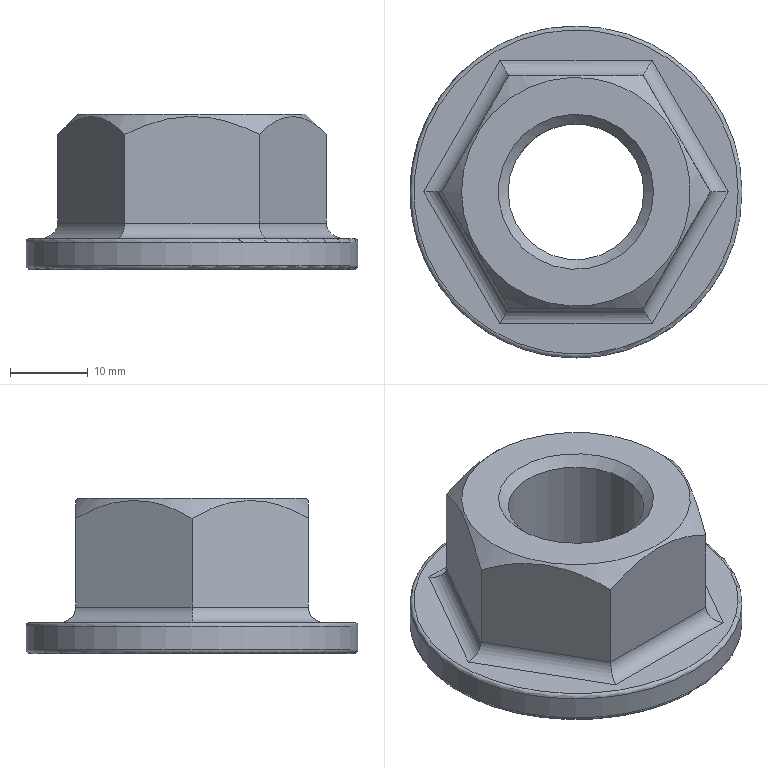Part | STEP file | YBQDJ-YB-10 | 1 solid | 22 faces | box 42.8 x 42.8 x 20 mm | volume 13331 mm3 | plane 9 | cylinder 8 | cone 3 | torus 2 | commonest cylinder face diameters 4 x6 17.5 x1 42.8 x1